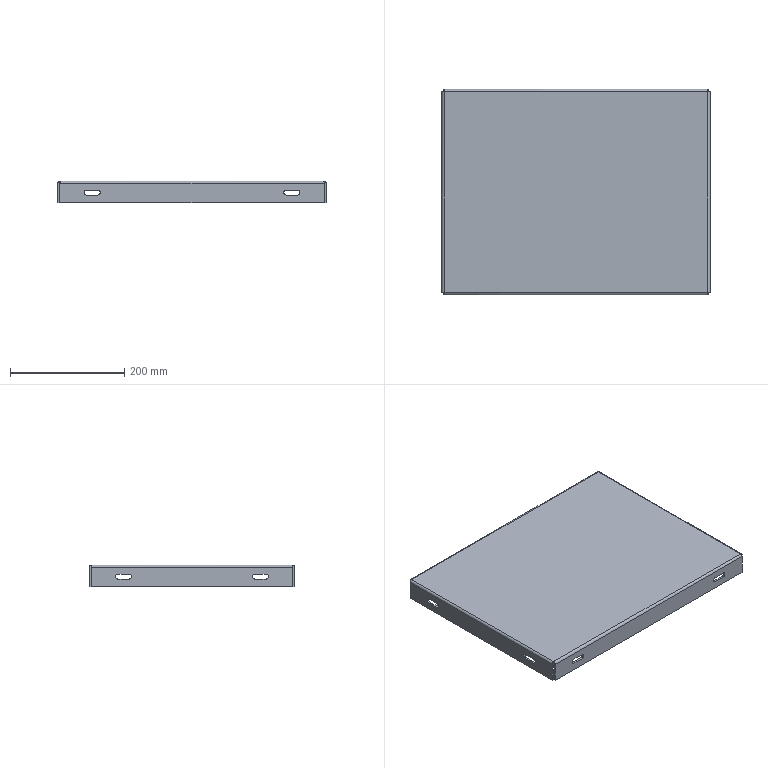Part | NX | features BREP 1 | 1 solid | 70 faces | box 469 x 359 x 38 mm | volume 665024 mm3 | plane 38 | cylinder 24 | spline 8 | commonest cylinder face diameters 8.5 x16 2 x4 8 x4